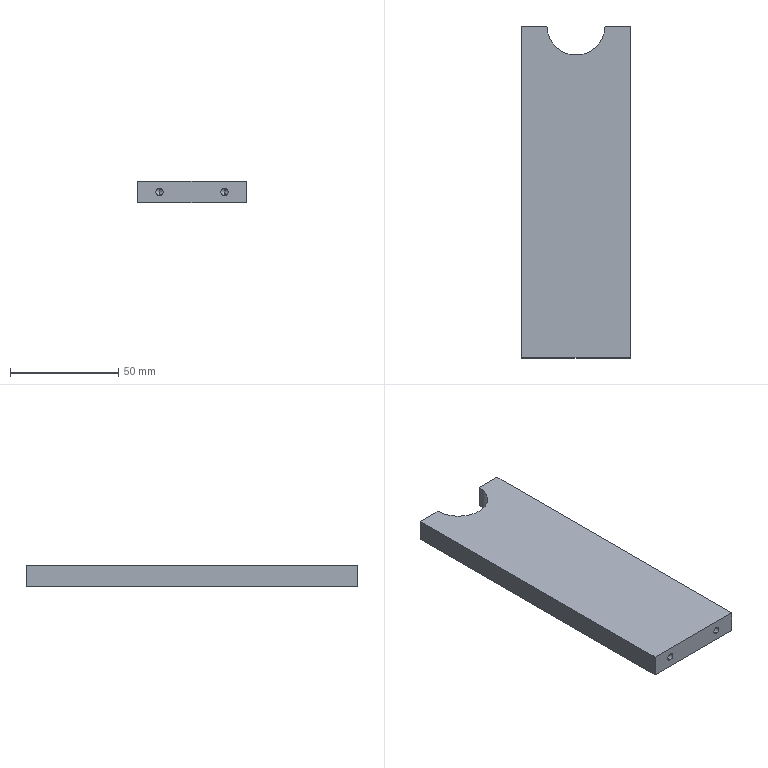Part | STEP file | 2095 Cylinder support plate | 1 solid | 24 faces | box 50 x 153 x 10 mm | volume 73275 mm3 | cylinder 9 | cone 8 | plane 7 | commonest cylinder face diameters 3.3 x8 26.8 x1